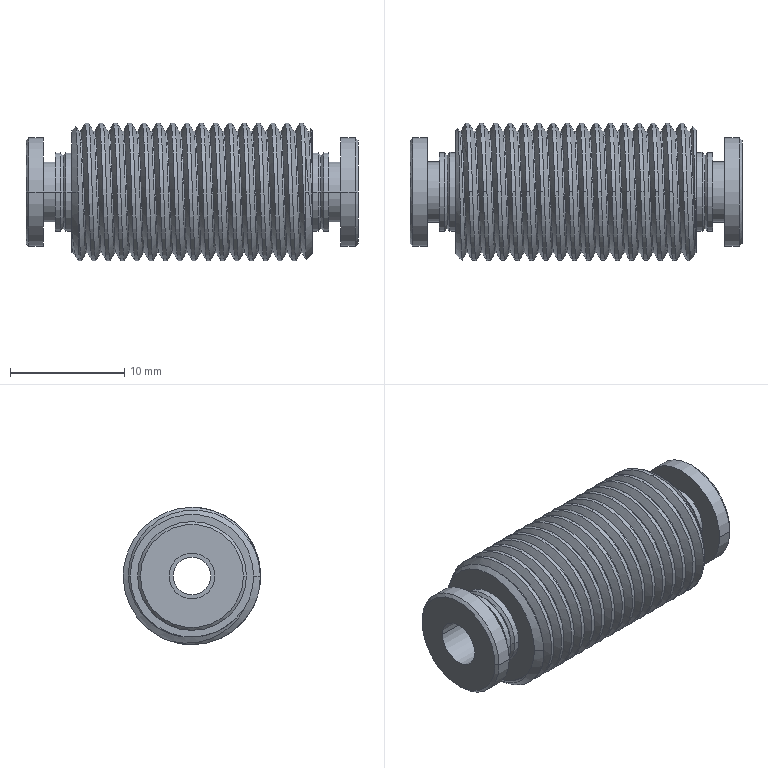Part | NX | features BREP 1 | 1 solid | 86 faces | box 29 x 12 x 12 mm | volume 2150 mm3 | cylinder 55 | cone 18 | plane 10 | spline 3 | commonest cylinder face diameters 12 x33 6.9 x8 4 x4 5.26 x4 9.5 x4 3.3 x2